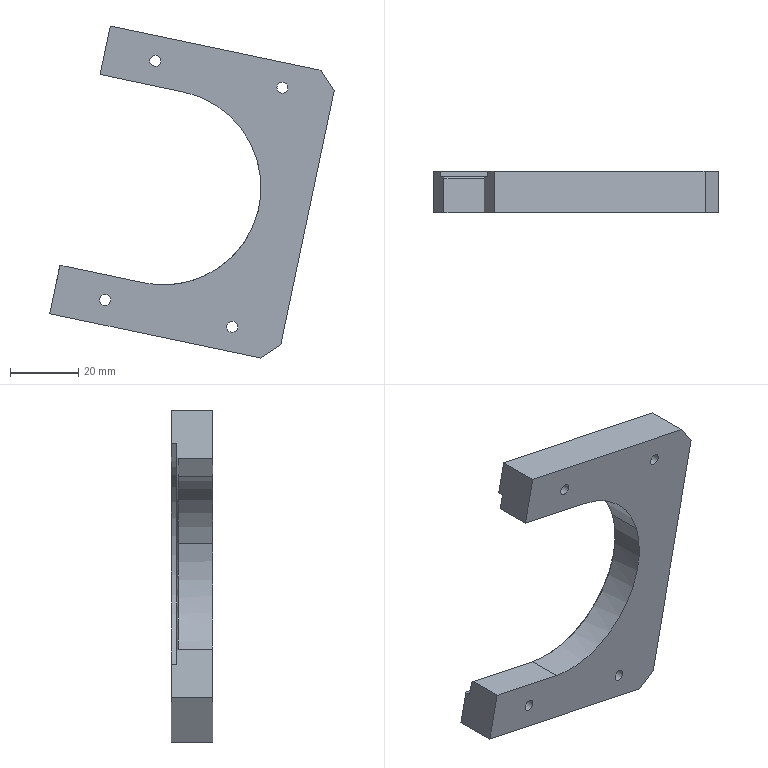Part | STEP file | BERCO_001 | 1 solid | 25 faces | box 83.204 x 12 x 97.117 mm | volume 36018 mm3 | plane 16 | cylinder 6 | spline 2 | cone 1 | commonest cylinder face diameters 3.242 x4 56.999 x1 66.1 x1